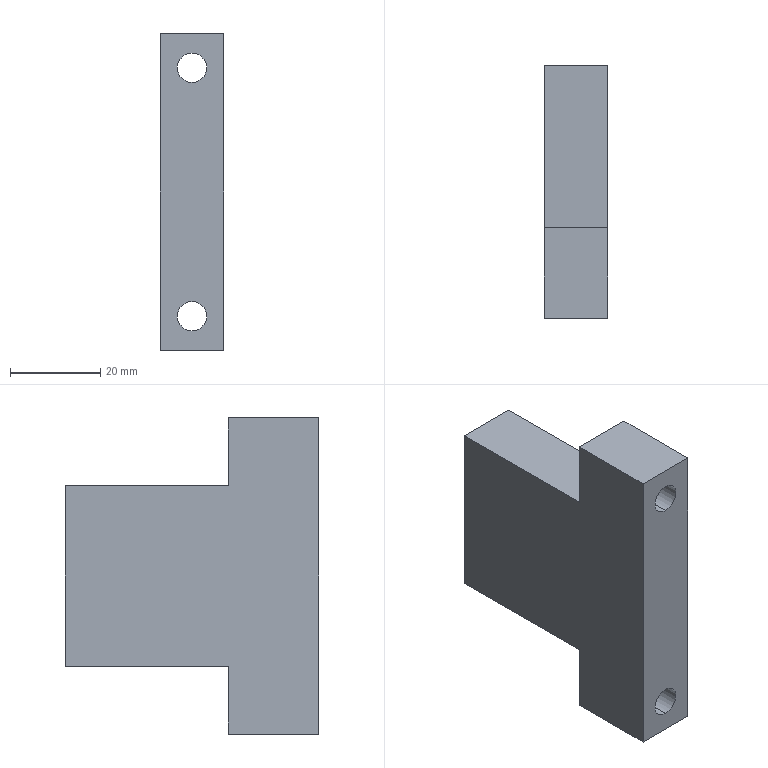Part | STEP file | PN_0057 cylinder spacer block | 1 solid | 22 faces | box 14 x 56 x 70 mm | volume 38077 mm3 | plane 10 | cylinder 8 | cone 4 | commonest cylinder face diameters 4.2 x4 6.5 x4